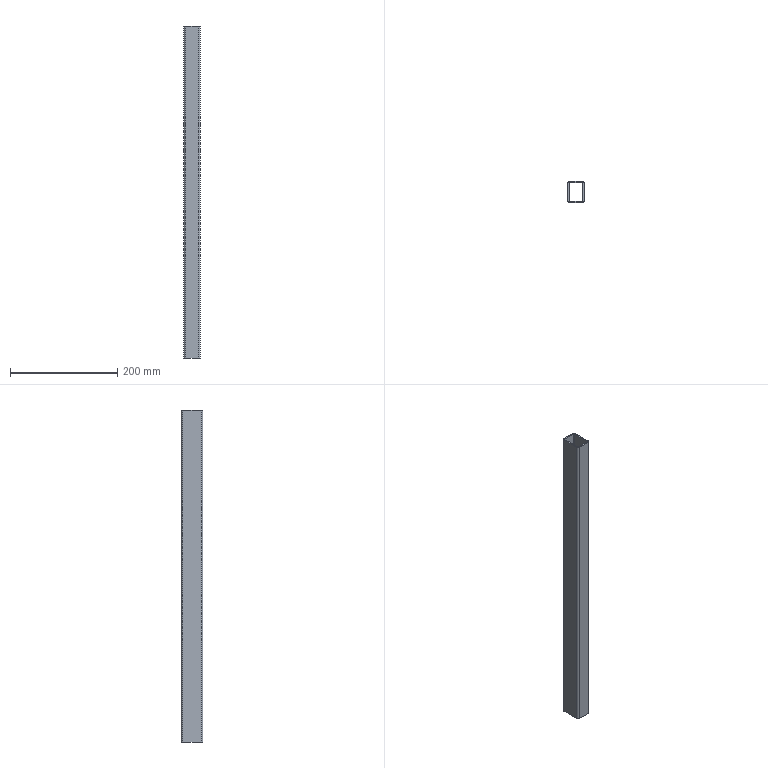Part | SolidWorks | features BaseBody 1 | 1 solid | 18 faces | box 30 x 40 x 620 mm | volume 196843 mm3 | plane 10 | cylinder 8 | commonest cylinder face diameters 1 x4 6 x4
STEP:
#1=CARTESIAN_POINT('',(12.,17.5,-310.));
#2=VERTEX_POINT('',#1);
#3=CARTESIAN_POINT('',(-12.,17.5,-310.));
#4=VERTEX_POINT('',#3);
#5=CARTESIAN_POINT('',(-12.,17.5,-310.));
#6=DIRECTION('',(-1.,0.,0.));
#7=VECTOR('',#6,1000.);
#8=LINE('',#5,#7);
#9=EDGE_CURVE('',#2,#4,#8,.T.);
#10=ORIENTED_EDGE('',*,*,#9,.F.);
#11=CARTESIAN_POINT('',(12.,17.5,310.));
#12=VERTEX_POINT('',#11);
#13=CARTESIAN_POINT('',(12.,17.5,310.));
#14=DIRECTION('',(0.,0.,-1.));
#15=VECTOR('',#14,1000.);
#16=LINE('',#13,#15);
#17=EDGE_CURVE('',#12,#2,#16,.T.);
#18=ORIENTED_EDGE('',*,*,#17,.F.);
#19=CARTESIAN_POINT('',(-12.,17.5,310.));
#20=VERTEX_POINT('',#19);
#21=CARTESIAN_POINT('',(-12.,17.5,310.));
#22=DIRECTION('',(-1.,0.,0.));
#23=VECTOR('',#22,1000.);
#24=LINE('',#21,#23);
#25=EDGE_CURVE('',#12,#20,#24,.T.);
#26=ORIENTED_EDGE('',*,*,#25,.T.);
#27=CARTESIAN_POINT('',(-12.,17.5,310.));
#28=DIRECTION('',(0.,0.,-1.));
#29=VECTOR('',#28,1000.);
#30=LINE('',#27,#29);
#31=EDGE_CURVE('',#20,#4,#30,.T.);
#32=ORIENTED_EDGE('',*,*,#31,.T.);
#33=EDGE_LOOP('',(#10,#18,#26,#32));
#34=FACE_OUTER_BOUND('',#33,.T.);
#35=CARTESIAN_POINT('',(-12.,17.5,310.));
#36=DIRECTION('',(0.,-1.,0.));
#37=DIRECTION('',(0.,0.,-1.));
#38=AXIS2_PLACEMENT_3D('',#35,#36,#37);
#39=PLANE('',#38);
#40=ADVANCED_FACE('',(#34),#39,.T.);
#41=CARTESIAN_POINT('',(12.5,17.,-310.));
#42=VERTEX_POINT('',#41);
#43=CARTESIAN_POINT('',(12.,17.,-310.));
#44=DIRECTION('',(0.,0.,1.));
#45=DIRECTION('',(-1.,0.,0.));
#46=AXIS2_PLACEMENT_3D('',#43,#44,#45);
#47=CIRCLE('',#46,0.5);
#48=EDGE_CURVE('',#42,#2,#47,.T.);
#49=ORIENTED_EDGE('',*,*,#48,.F.);
#50=CARTESIAN_POINT('',(12.5,17.,310.));
#51=VERTEX_POINT('',#50);
#52=CARTESIAN_POINT('',(12.5,17.,310.));
#53=DIRECTION('',(0.,0.,-1.));
#54=VECTOR('',#53,1000.);
#55=LINE('',#52,#54);
#56=EDGE_CURVE('',#51,#42,#55,.T.);
#57=ORIENTED_EDGE('',*,*,#56,.F.);
#58=CARTESIAN_POINT('',(12.,17.,310.));
#59=DIRECTION('',(0.,0.,1.));
#60=DIRECTION('',(-1.,0.,0.));
#61=AXIS2_PLACEMENT_3D('',#58,#59,#60);
#62=CIRCLE('',#61,0.5);
#63=EDGE_CURVE('',#51,#12,#62,.T.);
#64=ORIENTED_EDGE('',*,*,#63,.T.);
#65=ORIENTED_EDGE('',*,*,#17,.T.);
#66=EDGE_LOOP('',(#49,#57,#64,#65));
#67=FACE_OUTER_BOUND('',#66,.T.);
#68=CARTESIAN_POINT('',(12.,17.,310.));
#69=DIRECTION('',(0.,0.,-1.));
#70=DIRECTION('',(-1.,0.,0.));
#71=AXIS2_PLACEMENT_3D('',#68,#69,#70);
#72=CYLINDRICAL_SURFACE('',#71,0.5);
#73=ADVANCED_FACE('',(#67),#72,.F.);
#74=CARTESIAN_POINT('',(12.5,-17.,-310.));
#75=VERTEX_POINT('',#74);
#76=CARTESIAN_POINT('',(12.5,17.,-310.));
#77=DIRECTION('',(0.,1.,0.));
#78=VECTOR('',#77,1000.);
#79=LINE('',#76,#78);
#80=EDGE_CURVE('',#75,#42,#79,.T.);
#81=ORIENTED_EDGE('',*,*,#80,.F.);
#82=CARTESIAN_POINT('',(12.5,-17.,310.));
#83=VERTEX_POINT('',#82);
#84=CARTESIAN_POINT('',(12.5,-17.,310.));
#85=DIRECTION('',(0.,0.,-1.));
#86=VECTOR('',#85,1000.);
#87=LINE('',#84,#86);
#88=EDGE_CURVE('',#83,#75,#87,.T.);
#89=ORIENTED_EDGE('',*,*,#88,.F.);
#90=CARTESIAN_POINT('',(12.5,17.,310.));
#91=DIRECTION('',(0.,1.,0.));
#92=VECTOR('',#91,1000.);
#93=LINE('',#90,#92);
#94=EDGE_CURVE('',#83,#51,#93,.T.);
#95=ORIENTED_EDGE('',*,*,#94,.T.);
#96=ORIENTED_EDGE('',*,*,#56,.T.);
#97=EDGE_LOOP('',(#81,#89,#95,#96));
#98=FACE_OUTER_BOUND('',#97,.T.);
#99=CARTESIAN_POINT('',(12.5,17.,310.));
#100=DIRECTION('',(-1.,0.,0.));
#101=DIRECTION('',(0.,1.,0.));
#102=AXIS2_PLACEMENT_3D('',#99,#100,#101);
#103=PLANE('',#102);
#104=ADVANCED_FACE('',(#98),#103,.T.);
#105=CARTESIAN_POINT('',(12.,-17.5,-310.));
#106=VERTEX_POINT('',#105);
#107=CARTESIAN_POINT('',(12.,-17.,-310.));
#108=DIRECTION('',(0.,0.,1.));
#109=DIRECTION('',(1.,0.,0.));
#110=AXIS2_PLACEMENT_3D('',#107,#108,#109);
#111=CIRCLE('',#110,0.5);
#112=EDGE_CURVE('',#106,#75,#111,.T.);
#113=ORIENTED_EDGE('',*,*,#112,.F.);
#114=CARTESIAN_POINT('',(12.,-17.5,310.));
#115=VERTEX_POINT('',#114);
#116=CARTESIAN_POINT('',(12.,-17.5,310.));
#117=DIRECTION('',(0.,0.,-1.));
#118=VECTOR('',#117,1000.);
#119=LINE('',#116,#118);
#120=EDGE_CURVE('',#115,#106,#119,.T.);
#121=ORIENTED_EDGE('',*,*,#120,.F.);
#122=CARTESIAN_POINT('',(12.,-17.,310.));
#123=DIRECTION('',(0.,0.,1.));
#124=DIRECTION('',(1.,0.,0.));
#125=AXIS2_PLACEMENT_3D('',#122,#123,#124);
#126=CIRCLE('',#125,0.5);
#127=EDGE_CURVE('',#115,#83,#126,.T.);
#128=ORIENTED_EDGE('',*,*,#127,.T.);
#129=ORIENTED_EDGE('',*,*,#88,.T.);
#130=EDGE_LOOP('',(#113,#121,#128,#129));
#131=FACE_OUTER_BOUND('',#130,.T.);
#132=CARTESIAN_POINT('',(12.,-17.,310.));
#133=DIRECTION('',(0.,0.,-1.));
#134=DIRECTION('',(-1.,0.,0.));
#135=AXIS2_PLACEMENT_3D('',#132,#133,#134);
#136=CYLINDRICAL_SURFACE('',#135,0.5);
#137=ADVANCED_FACE('',(#131),#136,.F.);
#138=CARTESIAN_POINT('',(-12.,-17.5,-310.));
#139=VERTEX_POINT('',#138);
#140=CARTESIAN_POINT('',(-12.,-17.5,-310.));
#141=DIRECTION('',(1.,0.,0.));
#142=VECTOR('',#141,1000.);
#143=LINE('',#140,#142);
#144=EDGE_CURVE('',#139,#106,#143,.T.);
#145=ORIENTED_EDGE('',*,*,#144,.F.);
#146=CARTESIAN_POINT('',(-12.,-17.5,310.));
#147=VERTEX_POINT('',#146);
#148=CARTESIAN_POINT('',(-12.,-17.5,310.));
#149=DIRECTION('',(0.,0.,-1.));
#150=VECTOR('',#149,1000.);
#151=LINE('',#148,#150);
#152=EDGE_CURVE('',#147,#139,#151,.T.);
#153=ORIENTED_EDGE('',*,*,#152,.F.);
#154=CARTESIAN_POINT('',(-12.,-17.5,310.));
#155=DIRECTION('',(1.,0.,0.));
#156=VECTOR('',#155,1000.);
#157=LINE('',#154,#156);
#158=EDGE_CURVE('',#147,#115,#157,.T.);
#159=ORIENTED_EDGE('',*,*,#158,.T.);
#160=ORIENTED_EDGE('',*,*,#120,.T.);
#161=EDGE_LOOP('',(#145,#153,#159,#160));
#162=FACE_OUTER_BOUND('',#161,.T.);
#163=CARTESIAN_POINT('',(-12.,-17.5,310.));
#164=DIRECTION('',(0.,1.,0.));
#165=DIRECTION('',(1.,0.,0.));
#166=AXIS2_PLACEMENT_3D('',#163,#164,#165);
#167=PLANE('',#166);
#168=ADVANCED_FACE('',(#162),#167,.T.);
#169=CARTESIAN_POINT('',(-12.5,-17.,-310.));
#170=VERTEX_POINT('',#169);
#171=CARTESIAN_POINT('',(-12.,-17.,-310.));
#172=DIRECTION('',(0.,0.,1.));
#173=DIRECTION('',(1.,0.,0.));
#174=AXIS2_PLACEMENT_3D('',#171,#172,#173);
#175=CIRCLE('',#174,0.5);
#176=EDGE_CURVE('',#170,#139,#175,.T.);
#177=ORIENTED_EDGE('',*,*,#176,.F.);
#178=CARTESIAN_POINT('',(-12.5,-17.,310.));
#179=VERTEX_POINT('',#178);
#180=CARTESIAN_POINT('',(-12.5,-17.,310.));
#181=DIRECTION('',(0.,0.,-1.));
#182=VECTOR('',#181,1000.);
#183=LINE('',#180,#182);
#184=EDGE_CURVE('',#179,#170,#183,.T.);
#185=ORIENTED_EDGE('',*,*,#184,.F.);
#186=CARTESIAN_POINT('',(-12.,-17.,310.));
#187=DIRECTION('',(0.,0.,1.));
#188=DIRECTION('',(1.,0.,0.));
#189=AXIS2_PLACEMENT_3D('',#186,#187,#188);
#190=CIRCLE('',#189,0.5);
#191=EDGE_CURVE('',#179,#147,#190,.T.);
#192=ORIENTED_EDGE('',*,*,#191,.T.);
#193=ORIENTED_EDGE('',*,*,#152,.T.);
#194=EDGE_LOOP('',(#177,#185,#192,#193));
#195=FACE_OUTER_BOUND('',#194,.T.);
#196=CARTESIAN_POINT('',(-12.,-17.,310.));
#197=DIRECTION('',(0.,0.,-1.));
#198=DIRECTION('',(-1.,0.,0.));
#199=AXIS2_PLACEMENT_3D('',#196,#197,#198);
#200=CYLINDRICAL_SURFACE('',#199,0.5);
#201=ADVANCED_FACE('',(#195),#200,.F.);
#202=CARTESIAN_POINT('',(-12.5,17.,-310.));
#203=VERTEX_POINT('',#202);
#204=CARTESIAN_POINT('',(-12.5,17.,-310.));
#205=DIRECTION('',(0.,-1.,0.));
#206=VECTOR('',#205,1000.);
#207=LINE('',#204,#206);
#208=EDGE_CURVE('',#203,#170,#207,.T.);
#209=ORIENTED_EDGE('',*,*,#208,.F.);
#210=CARTESIAN_POINT('',(-12.5,17.,310.));
#211=VERTEX_POINT('',#210);
#212=CARTESIAN_POINT('',(-12.5,17.,310.));
#213=DIRECTION('',(0.,0.,-1.));
#214=VECTOR('',#213,1000.);
#215=LINE('',#212,#214);
#216=EDGE_CURVE('',#211,#203,#215,.T.);
#217=ORIENTED_EDGE('',*,*,#216,.F.);
#218=CARTESIAN_POINT('',(-12.5,17.,310.));
#219=DIRECTION('',(0.,-1.,0.));
#220=VECTOR('',#219,1000.);
#221=LINE('',#218,#220);
#222=EDGE_CURVE('',#211,#179,#221,.T.);
#223=ORIENTED_EDGE('',*,*,#222,.T.);
#224=ORIENTED_EDGE('',*,*,#184,.T.);
#225=EDGE_LOOP('',(#209,#217,#223,#224));
#226=FACE_OUTER_BOUND('',#225,.T.);
#227=CARTESIAN_POINT('',(-12.5,17.,310.));
#228=DIRECTION('',(1.,0.,0.));
#229=DIRECTION('',(0.,1.,0.));
#230=AXIS2_PLACEMENT_3D('',#227,#228,#229);
#231=PLANE('',#230);
#232=ADVANCED_FACE('',(#226),#231,.T.);
#233=CARTESIAN_POINT('',(-12.,17.,-310.));
#234=DIRECTION('',(0.,0.,1.));
#235=DIRECTION('',(1.,0.,0.));
#236=AXIS2_PLACEMENT_3D('',#233,#234,#235);
#237=CIRCLE('',#236,0.5);
#238=EDGE_CURVE('',#4,#203,#237,.T.);
#239=ORIENTED_EDGE('',*,*,#238,.F.);
#240=ORIENTED_EDGE('',*,*,#31,.F.);
#241=CARTESIAN_POINT('',(-12.,17.,310.));
#242=DIRECTION('',(0.,0.,1.));
#243=DIRECTION('',(1.,0.,0.));
#244=AXIS2_PLACEMENT_3D('',#241,#242,#243);
#245=CIRCLE('',#244,0.5);
#246=EDGE_CURVE('',#20,#211,#245,.T.);
#247=ORIENTED_EDGE('',*,*,#246,.T.);
#248=ORIENTED_EDGE('',*,*,#216,.T.);
#249=EDGE_LOOP('',(#239,#240,#247,#248));
#250=FACE_OUTER_BOUND('',#249,.T.);
#251=CARTESIAN_POINT('',(-12.,17.,310.));
#252=DIRECTION('',(0.,0.,-1.));
#253=DIRECTION('',(-1.,0.,0.));
#254=AXIS2_PLACEMENT_3D('',#251,#252,#253);
#255=CYLINDRICAL_SURFACE('',#254,0.5);
#256=ADVANCED_FACE('',(#250),#255,.F.);
#257=CARTESIAN_POINT('',(-15.,17.,-310.));
#258=VERTEX_POINT('',#257);
#259=CARTESIAN_POINT('',(-15.,-17.,-310.));
#260=VERTEX_POINT('',#259);
#261=CARTESIAN_POINT('',(-15.,17.,-310.));
#262=DIRECTION('',(0.,-1.,0.));
#263=VECTOR('',#262,1000.);
#264=LINE('',#261,#263);
#265=EDGE_CURVE('',#258,#260,#264,.T.);
#266=ORIENTED_EDGE('',*,*,#265,.T.);
#267=CARTESIAN_POINT('',(-15.,-17.,310.));
#268=VERTEX_POINT('',#267);
#269=CARTESIAN_POINT('',(-15.,-17.,310.));
#270=DIRECTION('',(0.,0.,-1.));
#271=VECTOR('',#270,1000.);
#272=LINE('',#269,#271);
#273=EDGE_CURVE('',#268,#260,#272,.T.);
#274=ORIENTED_EDGE('',*,*,#273,.F.);
#275=CARTESIAN_POINT('',(-15.,17.,310.));
#276=VERTEX_POINT('',#275);
#277=CARTESIAN_POINT('',(-15.,17.,310.));
#278=DIRECTION('',(0.,-1.,0.));
#279=VECTOR('',#278,1000.);
#280=LINE('',#277,#279);
#281=EDGE_CURVE('',#276,#268,#280,.T.);
#282=ORIENTED_EDGE('',*,*,#281,.F.);
#283=CARTESIAN_POINT('',(-15.,17.,310.));
#284=DIRECTION('',(0.,0.,-1.));
#285=VECTOR('',#284,1000.);
#286=LINE('',#283,#285);
#287=EDGE_CURVE('',#276,#258,#286,.T.);
#288=ORIENTED_EDGE('',*,*,#287,.T.);
#289=EDGE_LOOP('',(#266,#274,#282,#288));
#290=FACE_OUTER_BOUND('',#289,.T.);
#291=CARTESIAN_POINT('',(-15.,17.,310.));
#292=DIRECTION('',(1.,0.,0.));
#293=DIRECTION('',(0.,1.,0.));
#294=AXIS2_PLACEMENT_3D('',#291,#292,#293);
#295=PLANE('',#294);
#296=ADVANCED_FACE('',(#290),#295,.F.);
#297=CARTESIAN_POINT('',(-12.,20.,-310.));
#298=VERTEX_POINT('',#297);
#299=CARTESIAN_POINT('',(-12.,17.,-310.));
#300=DIRECTION('',(0.,0.,1.));
#301=DIRECTION('',(1.,0.,0.));
#302=AXIS2_PLACEMENT_3D('',#299,#300,#301);
#303=CIRCLE('',#302,3.);
#304=EDGE_CURVE('',#298,#258,#303,.T.);
#305=ORIENTED_EDGE('',*,*,#304,.T.);
#306=ORIENTED_EDGE('',*,*,#287,.F.);
#307=CARTESIAN_POINT('',(-12.,20.,310.));
#308=VERTEX_POINT('',#307);
#309=CARTESIAN_POINT('',(-12.,17.,310.));
#310=DIRECTION('',(0.,0.,1.));
#311=DIRECTION('',(1.,0.,0.));
#312=AXIS2_PLACEMENT_3D('',#309,#310,#311);
#313=CIRCLE('',#312,3.);
#314=EDGE_CURVE('',#308,#276,#313,.T.);
#315=ORIENTED_EDGE('',*,*,#314,.F.);
#316=CARTESIAN_POINT('',(-12.,20.,310.));
#317=DIRECTION('',(0.,0.,-1.));
#318=VECTOR('',#317,1000.);
#319=LINE('',#316,#318);
#320=EDGE_CURVE('',#308,#298,#319,.T.);
#321=ORIENTED_EDGE('',*,*,#320,.T.);
#322=EDGE_LOOP('',(#305,#306,#315,#321));
#323=FACE_OUTER_BOUND('',#322,.T.);
#324=CARTESIAN_POINT('',(-12.,17.,310.));
#325=DIRECTION('',(0.,0.,-1.));
#326=DIRECTION('',(-1.,0.,0.));
#327=AXIS2_PLACEMENT_3D('',#324,#325,#326);
#328=CYLINDRICAL_SURFACE('',#327,3.);
#329=ADVANCED_FACE('',(#323),#328,.T.);
#330=CARTESIAN_POINT('',(12.,20.,-310.));
#331=VERTEX_POINT('',#330);
#332=CARTESIAN_POINT('',(-12.,20.,-310.));
#333=DIRECTION('',(-1.,0.,0.));
#334=VECTOR('',#333,1000.);
#335=LINE('',#332,#334);
#336=EDGE_CURVE('',#331,#298,#335,.T.);
#337=ORIENTED_EDGE('',*,*,#336,.T.);
#338=ORIENTED_EDGE('',*,*,#320,.F.);
#339=CARTESIAN_POINT('',(12.,20.,310.));
#340=VERTEX_POINT('',#339);
#341=CARTESIAN_POINT('',(-12.,20.,310.));
#342=DIRECTION('',(-1.,0.,0.));
#343=VECTOR('',#342,1000.);
#344=LINE('',#341,#343);
#345=EDGE_CURVE('',#340,#308,#344,.T.);
#346=ORIENTED_EDGE('',*,*,#345,.F.);
#347=CARTESIAN_POINT('',(12.,20.,310.));
#348=DIRECTION('',(0.,0.,-1.));
#349=VECTOR('',#348,1000.);
#350=LINE('',#347,#349);
#351=EDGE_CURVE('',#340,#331,#350,.T.);
#352=ORIENTED_EDGE('',*,*,#351,.T.);
#353=EDGE_LOOP('',(#337,#338,#346,#352));
#354=FACE_OUTER_BOUND('',#353,.T.);
#355=CARTESIAN_POINT('',(-12.,20.,310.));
#356=DIRECTION('',(0.,-1.,0.));
#357=DIRECTION('',(0.,0.,-1.));
#358=AXIS2_PLACEMENT_3D('',#355,#356,#357);
#359=PLANE('',#358);
#360=ADVANCED_FACE('',(#354),#359,.F.);
#361=CARTESIAN_POINT('',(15.,17.,-310.));
#362=VERTEX_POINT('',#361);
#363=CARTESIAN_POINT('',(12.,17.,-310.));
#364=DIRECTION('',(0.,0.,1.));
#365=DIRECTION('',(-1.,0.,0.));
#366=AXIS2_PLACEMENT_3D('',#363,#364,#365);
#367=CIRCLE('',#366,3.);
#368=EDGE_CURVE('',#362,#331,#367,.T.);
#369=ORIENTED_EDGE('',*,*,#368,.T.);
#370=ORIENTED_EDGE('',*,*,#351,.F.);
#371=CARTESIAN_POINT('',(15.,17.,310.));
#372=VERTEX_POINT('',#371);
#373=CARTESIAN_POINT('',(12.,17.,310.));
#374=DIRECTION('',(0.,0.,1.));
#375=DIRECTION('',(-1.,0.,0.));
#376=AXIS2_PLACEMENT_3D('',#373,#374,#375);
#377=CIRCLE('',#376,3.);
#378=EDGE_CURVE('',#372,#340,#377,.T.);
#379=ORIENTED_EDGE('',*,*,#378,.F.);
#380=CARTESIAN_POINT('',(15.,17.,310.));
#381=DIRECTION('',(0.,0.,-1.));
#382=VECTOR('',#381,1000.);
#383=LINE('',#380,#382);
#384=EDGE_CURVE('',#372,#362,#383,.T.);
#385=ORIENTED_EDGE('',*,*,#384,.T.);
#386=EDGE_LOOP('',(#369,#370,#379,#385));
#387=FACE_OUTER_BOUND('',#386,.T.);
#388=CARTESIAN_POINT('',(12.,17.,310.));
#389=DIRECTION('',(0.,0.,-1.));
#390=DIRECTION('',(-1.,0.,0.));
#391=AXIS2_PLACEMENT_3D('',#388,#389,#390);
#392=CYLINDRICAL_SURFACE('',#391,3.);
#393=ADVANCED_FACE('',(#387),#392,.T.);
#394=CARTESIAN_POINT('',(15.,-17.,-310.));
#395=VERTEX_POINT('',#394);
#396=CARTESIAN_POINT('',(15.,17.,-310.));
#397=DIRECTION('',(0.,1.,0.));
#398=VECTOR('',#397,1000.);
#399=LINE('',#396,#398);
#400=EDGE_CURVE('',#395,#362,#399,.T.);
#401=ORIENTED_EDGE('',*,*,#400,.T.);
#402=ORIENTED_EDGE('',*,*,#384,.F.);
#403=CARTESIAN_POINT('',(15.,-17.,310.));
#404=VERTEX_POINT('',#403);
#405=CARTESIAN_POINT('',(15.,17.,310.));
#406=DIRECTION('',(0.,1.,0.));
#407=VECTOR('',#406,1000.);
#408=LINE('',#405,#407);
#409=EDGE_CURVE('',#404,#372,#408,.T.);
#410=ORIENTED_EDGE('',*,*,#409,.F.);
#411=CARTESIAN_POINT('',(15.,-17.,310.));
#412=DIRECTION('',(0.,0.,-1.));
#413=VECTOR('',#412,1000.);
#414=LINE('',#411,#413);
#415=EDGE_CURVE('',#404,#395,#414,.T.);
#416=ORIENTED_EDGE('',*,*,#415,.T.);
#417=EDGE_LOOP('',(#401,#402,#410,#416));
#418=FACE_OUTER_BOUND('',#417,.T.);
#419=CARTESIAN_POINT('',(15.,17.,310.));
#420=DIRECTION('',(-1.,0.,0.));
#421=DIRECTION('',(0.,1.,0.));
#422=AXIS2_PLACEMENT_3D('',#419,#420,#421);
#423=PLANE('',#422);
#424=ADVANCED_FACE('',(#418),#423,.F.);
#425=CARTESIAN_POINT('',(12.,-20.,-310.));
#426=VERTEX_POINT('',#425);
#427=CARTESIAN_POINT('',(12.,-17.,-310.));
#428=DIRECTION('',(0.,0.,1.));
#429=DIRECTION('',(1.,0.,0.));
#430=AXIS2_PLACEMENT_3D('',#427,#428,#429);
#431=CIRCLE('',#430,3.);
#432=EDGE_CURVE('',#426,#395,#431,.T.);
#433=ORIENTED_EDGE('',*,*,#432,.T.);
#434=ORIENTED_EDGE('',*,*,#415,.F.);
#435=CARTESIAN_POINT('',(12.,-20.,310.));
#436=VERTEX_POINT('',#435);
#437=CARTESIAN_POINT('',(12.,-17.,310.));
#438=DIRECTION('',(0.,0.,1.));
#439=DIRECTION('',(1.,0.,0.));
#440=AXIS2_PLACEMENT_3D('',#437,#438,#439);
#441=CIRCLE('',#440,3.);
#442=EDGE_CURVE('',#436,#404,#441,.T.);
#443=ORIENTED_EDGE('',*,*,#442,.F.);
#444=CARTESIAN_POINT('',(12.,-20.,310.));
#445=DIRECTION('',(0.,0.,-1.));
#446=VECTOR('',#445,1000.);
#447=LINE('',#444,#446);
#448=EDGE_CURVE('',#436,#426,#447,.T.);
#449=ORIENTED_EDGE('',*,*,#448,.T.);
#450=EDGE_LOOP('',(#433,#434,#443,#449));
#451=FACE_OUTER_BOUND('',#450,.T.);
#452=CARTESIAN_POINT('',(12.,-17.,310.));
#453=DIRECTION('',(0.,0.,-1.));
#454=DIRECTION('',(-1.,0.,0.));
#455=AXIS2_PLACEMENT_3D('',#452,#453,#454);
#456=CYLINDRICAL_SURFACE('',#455,3.);
#457=ADVANCED_FACE('',(#451),#456,.T.);
#458=CARTESIAN_POINT('',(-12.,-20.,-310.));
#459=VERTEX_POINT('',#458);
#460=CARTESIAN_POINT('',(-12.,-20.,-310.));
#461=DIRECTION('',(1.,0.,0.));
#462=VECTOR('',#461,1000.);
#463=LINE('',#460,#462);
#464=EDGE_CURVE('',#459,#426,#463,.T.);
#465=ORIENTED_EDGE('',*,*,#464,.T.);
#466=ORIENTED_EDGE('',*,*,#448,.F.);
#467=CARTESIAN_POINT('',(-12.,-20.,310.));
#468=VERTEX_POINT('',#467);
#469=CARTESIAN_POINT('',(-12.,-20.,310.));
#470=DIRECTION('',(1.,0.,0.));
#471=VECTOR('',#470,1000.);
#472=LINE('',#469,#471);
#473=EDGE_CURVE('',#468,#436,#472,.T.);
#474=ORIENTED_EDGE('',*,*,#473,.F.);
#475=CARTESIAN_POINT('',(-12.,-20.,310.));
#476=DIRECTION('',(0.,0.,-1.));
#477=VECTOR('',#476,1000.);
#478=LINE('',#475,#477);
#479=EDGE_CURVE('',#468,#459,#478,.T.);
#480=ORIENTED_EDGE('',*,*,#479,.T.);
#481=EDGE_LOOP('',(#465,#466,#474,#480));
#482=FACE_OUTER_BOUND('',#481,.T.);
#483=CARTESIAN_POINT('',(-12.,-20.,310.));
#484=DIRECTION('',(0.,1.,0.));
#485=DIRECTION('',(1.,0.,0.));
#486=AXIS2_PLACEMENT_3D('',#483,#484,#485);
#487=PLANE('',#486);
#488=ADVANCED_FACE('',(#482),#487,.F.);
#489=CARTESIAN_POINT('',(-12.,-17.,-310.));
#490=DIRECTION('',(0.,0.,1.));
#491=DIRECTION('',(1.,0.,0.));
#492=AXIS2_PLACEMENT_3D('',#489,#490,#491);
#493=CIRCLE('',#492,3.);
#494=EDGE_CURVE('',#260,#459,#493,.T.);
#495=ORIENTED_EDGE('',*,*,#494,.T.);
#496=ORIENTED_EDGE('',*,*,#479,.F.);
#497=CARTESIAN_POINT('',(-12.,-17.,310.));
#498=DIRECTION('',(0.,0.,1.));
#499=DIRECTION('',(1.,0.,0.));
#500=AXIS2_PLACEMENT_3D('',#497,#498,#499);
#501=CIRCLE('',#500,3.);
#502=EDGE_CURVE('',#268,#468,#501,.T.);
#503=ORIENTED_EDGE('',*,*,#502,.F.);
#504=ORIENTED_EDGE('',*,*,#273,.T.);
#505=EDGE_LOOP('',(#495,#496,#503,#504));
#506=FACE_OUTER_BOUND('',#505,.T.);
#507=CARTESIAN_POINT('',(-12.,-17.,310.));
#508=DIRECTION('',(0.,0.,-1.));
#509=DIRECTION('',(-1.,0.,0.));
#510=AXIS2_PLACEMENT_3D('',#507,#508,#509);
#511=CYLINDRICAL_SURFACE('',#510,3.);
#512=ADVANCED_FACE('',(#506),#511,.T.);
#513=ORIENTED_EDGE('',*,*,#238,.T.);
#514=ORIENTED_EDGE('',*,*,#208,.T.);
#515=ORIENTED_EDGE('',*,*,#176,.T.);
#516=ORIENTED_EDGE('',*,*,#144,.T.);
#517=ORIENTED_EDGE('',*,*,#112,.T.);
#518=ORIENTED_EDGE('',*,*,#80,.T.);
#519=ORIENTED_EDGE('',*,*,#48,.T.);
#520=ORIENTED_EDGE('',*,*,#9,.T.);
#521=EDGE_LOOP('',(#513,#514,#515,#516,#517,#518,#519,#520));
#522=FACE_BOUND('',#521,.T.);
#523=ORIENTED_EDGE('',*,*,#494,.F.);
#524=ORIENTED_EDGE('',*,*,#265,.F.);
#525=ORIENTED_EDGE('',*,*,#304,.F.);
#526=ORIENTED_EDGE('',*,*,#336,.F.);
#527=ORIENTED_EDGE('',*,*,#368,.F.);
#528=ORIENTED_EDGE('',*,*,#400,.F.);
#529=ORIENTED_EDGE('',*,*,#432,.F.);
#530=ORIENTED_EDGE('',*,*,#464,.F.);
#531=EDGE_LOOP('',(#523,#524,#525,#526,#527,#528,#529,#530));
#532=FACE_OUTER_BOUND('',#531,.T.);
#533=CARTESIAN_POINT('',(-12.,-17.,-310.));
#534=DIRECTION('',(0.,0.,1.));
#535=DIRECTION('',(1.,0.,0.));
#536=AXIS2_PLACEMENT_3D('',#533,#534,#535);
#537=PLANE('',#536);
#538=ADVANCED_FACE('',(#522,#532),#537,.F.);
#539=ORIENTED_EDGE('',*,*,#222,.F.);
#540=ORIENTED_EDGE('',*,*,#246,.F.);
#541=ORIENTED_EDGE('',*,*,#25,.F.);
#542=ORIENTED_EDGE('',*,*,#63,.F.);
#543=ORIENTED_EDGE('',*,*,#94,.F.);
#544=ORIENTED_EDGE('',*,*,#127,.F.);
#545=ORIENTED_EDGE('',*,*,#158,.F.);
#546=ORIENTED_EDGE('',*,*,#191,.F.);
#547=EDGE_LOOP('',(#539,#540,#541,#542,#543,#544,#545,#546));
#548=FACE_BOUND('',#547,.T.);
#549=ORIENTED_EDGE('',*,*,#502,.T.);
#550=ORIENTED_EDGE('',*,*,#473,.T.);
#551=ORIENTED_EDGE('',*,*,#442,.T.);
#552=ORIENTED_EDGE('',*,*,#409,.T.);
#553=ORIENTED_EDGE('',*,*,#378,.T.);
#554=ORIENTED_EDGE('',*,*,#345,.T.);
#555=ORIENTED_EDGE('',*,*,#314,.T.);
#556=ORIENTED_EDGE('',*,*,#281,.T.);
#557=EDGE_LOOP('',(#549,#550,#551,#552,#553,#554,#555,#556));
#558=FACE_OUTER_BOUND('',#557,.T.);
#559=CARTESIAN_POINT('',(-12.,-17.,310.));
#560=DIRECTION('',(0.,0.,1.));
#561=DIRECTION('',(1.,0.,0.));
#562=AXIS2_PLACEMENT_3D('',#559,#560,#561);
#563=PLANE('',#562);
#564=ADVANCED_FACE('',(#548,#558),#563,.T.);
#565=CLOSED_SHELL('',(#40,#73,#104,#137,#168,#201,#232,#256,#296,#329,#360,#393,#424,#457,#488,#512,#538,#564));
#566=MANIFOLD_SOLID_BREP('',#565);
#567=CARTESIAN_POINT('',(0.,0.,0.));
#568=DIRECTION('',(0.,0.,1.));
#569=DIRECTION('',(1.,0.,0.));
#570=AXIS2_PLACEMENT_3D('',#567,#568,#569);
#571=(LENGTH_UNIT()NAMED_UNIT(*)SI_UNIT(.MILLI.,.METRE.));
#572=UNCERTAINTY_MEASURE_WITH_UNIT(LENGTH_MEASURE(0.00001),#571,'','');
#573=(NAMED_UNIT(*)PLANE_ANGLE_UNIT()SI_UNIT($,.RADIAN.));
#574=(NAMED_UNIT(*)SI_UNIT($,.STERADIAN.)SOLID_ANGLE_UNIT());
#575=(GEOMETRIC_REPRESENTATION_CONTEXT(3)GLOBAL_UNCERTAINTY_ASSIGNED_CONTEXT((#572))GLOBAL_UNIT_ASSIGNED_CONTEXT((#571,#573,#574))REPRESENTATION_CONTEXT('',''));
#576=ADVANCED_BREP_SHAPE_REPRESENTATION('',(#566,#570),#575);